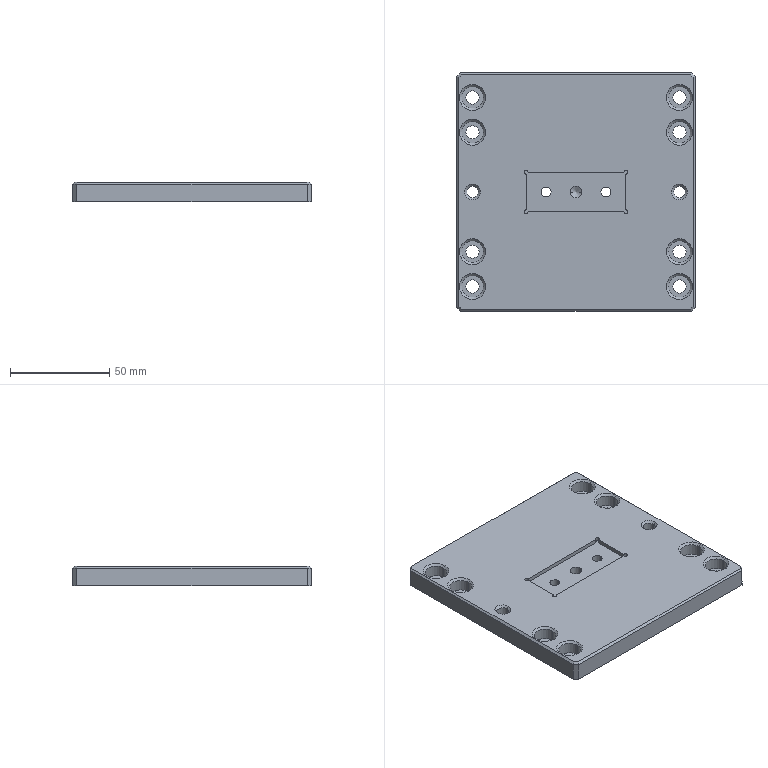Part | SolidWorks | features BaseBody 1 | 1 solid | 105 faces | box 120 x 120 x 10 mm | volume 134384 mm3 | cylinder 48 | plane 31 | cone 26 | commonest cylinder face diameters 6.6 x16 11 x16 2 x6 6 x6 5 x4